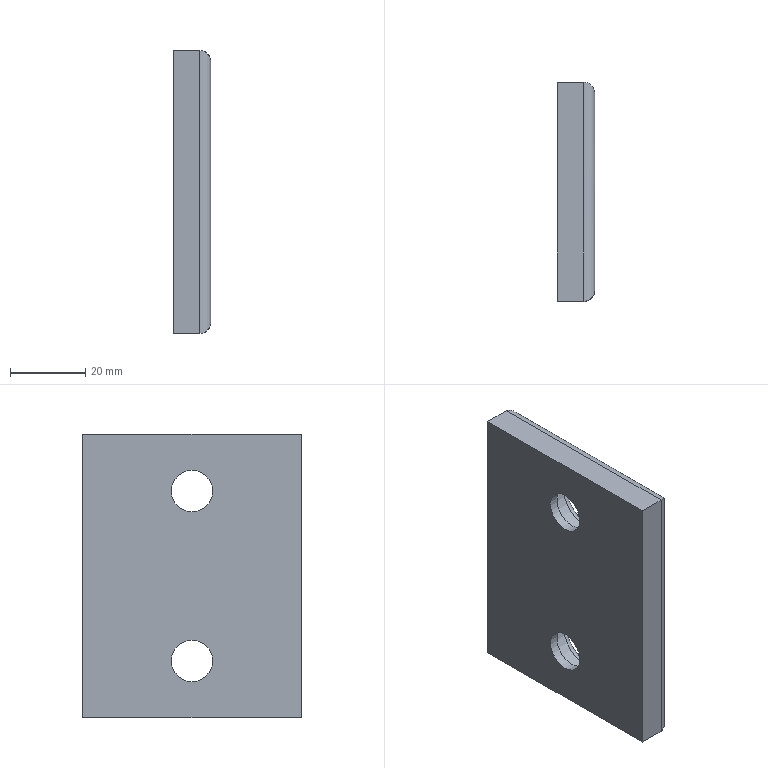Part | NX | features DB 2 | 1 solid | 144 faces | box 10 x 58 x 75 mm | volume 38808 mm3 | plane 99 | spline 35 | cylinder 8 | torus 2 | commonest cylinder face diameters 6 x4 11 x2 17.5 x2